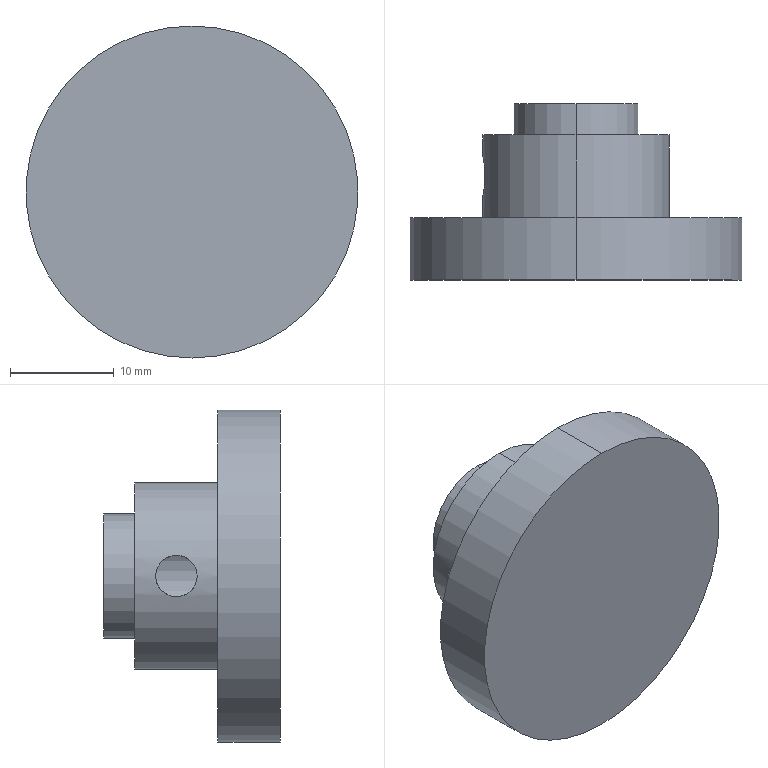Part | SolidWorks | features ICE 1, Revolution 1 | 1 solid | 15 faces | box 32 x 17 x 32 mm | volume 6483 mm3 | cylinder 10 | plane 5 | commonest cylinder face diameters 4 x2 8 x2 12 x2 18 x2 32 x2
STEP:
#1=CARTESIAN_POINT('',(-8.775,-3.306,-2.));
#2=VERTEX_POINT('',#1);
#3=CARTESIAN_POINT('',(-8.775,-3.306,2.));
#4=VERTEX_POINT('',#3);
#5=CARTESIAN_POINT('',(-8.775,-3.306,-2.));
#6=CARTESIAN_POINT('',(-8.775,-3.439,-2.));
#7=CARTESIAN_POINT('',(-8.778,-3.569,-1.987));
#8=CARTESIAN_POINT('',(-8.789,-3.826,-1.936));
#9=CARTESIAN_POINT('',(-8.798,-3.953,-1.897));
#10=CARTESIAN_POINT('',(-8.819,-4.195,-1.797));
#11=CARTESIAN_POINT('',(-8.831,-4.309,-1.735));
#12=CARTESIAN_POINT('',(-8.859,-4.527,-1.59));
#13=CARTESIAN_POINT('',(-8.874,-4.629,-1.506));
#14=CARTESIAN_POINT('',(-8.918,-4.905,-1.23));
#15=CARTESIAN_POINT('',(-8.947,-5.054,-1.007));
#16=CARTESIAN_POINT('',(-8.978,-5.203,-0.6467));
#17=CARTESIAN_POINT('',(-8.986,-5.242,-0.5202));
#18=CARTESIAN_POINT('',(-8.997,-5.294,-0.2618));
#19=CARTESIAN_POINT('',(-9.,-5.306,-0.1317));
#20=CARTESIAN_POINT('',(-9.,-5.306,0.1301));
#21=CARTESIAN_POINT('',(-8.997,-5.293,0.2631));
#22=CARTESIAN_POINT('',(-8.986,-5.242,0.52));
#23=CARTESIAN_POINT('',(-8.978,-5.204,0.6449));
#24=CARTESIAN_POINT('',(-8.947,-5.053,1.009));
#25=CARTESIAN_POINT('',(-8.918,-4.906,1.229));
#26=CARTESIAN_POINT('',(-8.873,-4.628,1.507));
#27=CARTESIAN_POINT('',(-8.859,-4.527,1.59));
#28=CARTESIAN_POINT('',(-8.832,-4.311,1.734));
#29=CARTESIAN_POINT('',(-8.819,-4.194,1.797));
#30=CARTESIAN_POINT('',(-8.798,-3.952,1.897));
#31=CARTESIAN_POINT('',(-8.789,-3.827,1.935));
#32=CARTESIAN_POINT('',(-8.778,-3.57,1.987));
#33=CARTESIAN_POINT('',(-8.775,-3.437,2.));
#34=CARTESIAN_POINT('',(-8.775,-3.306,2.));
#35=B_SPLINE_CURVE_WITH_KNOTS('',3,(#5,#6,#7,#8,#9,#10,#11,#12,#13,#14,#15,#16,#17,#18,#19,#20,#21,#22,#23,#24,#25,#26,#27,#28,#29,#30,#31,#32,#33,#34),.UNSPECIFIED.,.F.,.F.,(4,2,2,2,2,2,2,2,2,2,2,2,2,2,4),(0.,0.000392,0.0007841,0.001176,0.001568,0.002352,0.002744,0.003136,0.003528,0.00392,0.004704,0.005096,0.005488,0.00588,0.006273),.UNSPECIFIED.);
#36=EDGE_CURVE('',#2,#4,#35,.T.);
#37=ORIENTED_EDGE('',*,*,#36,.T.);
#38=CARTESIAN_POINT('',(-3.464,-3.306,2.));
#39=VERTEX_POINT('',#38);
#40=CARTESIAN_POINT('',(-10.,-3.306,2.));
#41=DIRECTION('',(1.,0.,0.));
#42=VECTOR('',#41,1000.);
#43=LINE('',#40,#42);
#44=EDGE_CURVE('',#4,#39,#43,.T.);
#45=ORIENTED_EDGE('',*,*,#44,.T.);
#46=CARTESIAN_POINT('',(-3.464,-3.306,-2.));
#47=VERTEX_POINT('',#46);
#48=CARTESIAN_POINT('',(-3.464,-3.306,2.));
#49=CARTESIAN_POINT('',(-3.464,-3.439,2.));
#50=CARTESIAN_POINT('',(-3.472,-3.574,1.986));
#51=CARTESIAN_POINT('',(-3.501,-3.833,1.934));
#52=CARTESIAN_POINT('',(-3.523,-3.958,1.895));
#53=CARTESIAN_POINT('',(-3.576,-4.201,1.794));
#54=CARTESIAN_POINT('',(-3.606,-4.315,1.732));
#55=CARTESIAN_POINT('',(-3.672,-4.529,1.588));
#56=CARTESIAN_POINT('',(-3.707,-4.63,1.505));
#57=CARTESIAN_POINT('',(-3.776,-4.811,1.324));
#58=CARTESIAN_POINT('',(-3.81,-4.893,1.225));
#59=CARTESIAN_POINT('',(-3.872,-5.038,1.01));
#60=CARTESIAN_POINT('',(-3.901,-5.1,0.8936));
#61=CARTESIAN_POINT('',(-3.972,-5.251,0.5337));
#62=CARTESIAN_POINT('',(-4.,-5.306,0.2665));
#63=CARTESIAN_POINT('',(-4.,-5.307,-0.1307));
#64=CARTESIAN_POINT('',(-3.993,-5.293,-0.265));
#65=CARTESIAN_POINT('',(-3.967,-5.241,-0.5254));
#66=CARTESIAN_POINT('',(-3.949,-5.202,-0.651));
#67=CARTESIAN_POINT('',(-3.877,-5.05,-1.015));
#68=CARTESIAN_POINT('',(-3.81,-4.902,-1.233));
#69=CARTESIAN_POINT('',(-3.707,-4.628,-1.507));
#70=CARTESIAN_POINT('',(-3.672,-4.529,-1.588));
#71=CARTESIAN_POINT('',(-3.607,-4.316,-1.732));
#72=CARTESIAN_POINT('',(-3.575,-4.2,-1.794));
#73=CARTESIAN_POINT('',(-3.523,-3.96,-1.895));
#74=CARTESIAN_POINT('',(-3.502,-3.835,-1.933));
#75=CARTESIAN_POINT('',(-3.472,-3.576,-1.986));
#76=CARTESIAN_POINT('',(-3.464,-3.441,-2.));
#77=CARTESIAN_POINT('',(-3.464,-3.306,-2.));
#78=B_SPLINE_CURVE_WITH_KNOTS('',3,(#48,#49,#50,#51,#52,#53,#54,#55,#56,#57,#58,#59,#60,#61,#62,#63,#64,#65,#66,#67,#68,#69,#70,#71,#72,#73,#74,#75,#76,#77),.UNSPECIFIED.,.F.,.F.,(4,2,2,2,2,2,2,2,2,2,2,2,2,2,4),(0.006361,0.006758,0.007155,0.007552,0.007949,0.008346,0.008742,0.009536,0.009933,0.01033,0.01112,0.01152,0.01192,0.01231,0.01271),.UNSPECIFIED.);
#79=EDGE_CURVE('',#39,#47,#78,.T.);
#80=ORIENTED_EDGE('',*,*,#79,.T.);
#81=CARTESIAN_POINT('',(-10.,-3.306,-2.));
#82=DIRECTION('',(1.,0.,0.));
#83=VECTOR('',#82,1000.);
#84=LINE('',#81,#83);
#85=EDGE_CURVE('',#2,#47,#84,.T.);
#86=ORIENTED_EDGE('',*,*,#85,.F.);
#87=EDGE_LOOP('',(#37,#45,#80,#86));
#88=FACE_OUTER_BOUND('',#87,.T.);
#89=CARTESIAN_POINT('',(-10.,-3.306,0.));
#90=DIRECTION('',(1.,0.,0.));
#91=DIRECTION('',(0.,0.,-1.));
#92=AXIS2_PLACEMENT_3D('',#89,#90,#91);
#93=CYLINDRICAL_SURFACE('',#92,2.);
#94=ADVANCED_FACE('',(#88),#93,.F.);
#95=CARTESIAN_POINT('',(0.,3.694,-6.));
#96=VERTEX_POINT('',#95);
#97=CARTESIAN_POINT('',(0.,3.694,6.));
#98=VERTEX_POINT('',#97);
#99=CARTESIAN_POINT('',(0.,3.694,0.));
#100=DIRECTION('',(0.,-1.,0.));
#101=DIRECTION('',(0.,0.,-1.));
#102=AXIS2_PLACEMENT_3D('',#99,#100,#101);
#103=CIRCLE('',#102,6.);
#104=EDGE_CURVE('',#96,#98,#103,.T.);
#105=ORIENTED_EDGE('',*,*,#104,.T.);
#106=CARTESIAN_POINT('',(0.,0.6936,6.));
#107=VERTEX_POINT('',#106);
#108=CARTESIAN_POINT('',(0.,0.,6.));
#109=DIRECTION('',(0.,-1.,0.));
#110=VECTOR('',#109,1000.);
#111=LINE('',#108,#110);
#112=EDGE_CURVE('',#98,#107,#111,.T.);
#113=ORIENTED_EDGE('',*,*,#112,.T.);
#114=CARTESIAN_POINT('',(0.,0.6936,-6.));
#115=VERTEX_POINT('',#114);
#116=CARTESIAN_POINT('',(0.,0.6936,0.));
#117=DIRECTION('',(0.,-1.,0.));
#118=DIRECTION('',(0.,0.,-1.));
#119=AXIS2_PLACEMENT_3D('',#116,#117,#118);
#120=CIRCLE('',#119,6.);
#121=EDGE_CURVE('',#115,#107,#120,.T.);
#122=ORIENTED_EDGE('',*,*,#121,.F.);
#123=CARTESIAN_POINT('',(0.,0.,-6.));
#124=DIRECTION('',(0.,-1.,0.));
#125=VECTOR('',#124,1000.);
#126=LINE('',#123,#125);
#127=EDGE_CURVE('',#96,#115,#126,.T.);
#128=ORIENTED_EDGE('',*,*,#127,.F.);
#129=EDGE_LOOP('',(#105,#113,#122,#128));
#130=FACE_OUTER_BOUND('',#129,.T.);
#131=CARTESIAN_POINT('',(0.,0.,0.));
#132=DIRECTION('',(0.,-1.,0.));
#133=DIRECTION('',(0.,0.,-1.));
#134=AXIS2_PLACEMENT_3D('',#131,#132,#133);
#135=CYLINDRICAL_SURFACE('',#134,6.);
#136=ADVANCED_FACE('',(#130),#135,.T.);
#137=CARTESIAN_POINT('',(0.,0.6936,-9.));
#138=VERTEX_POINT('',#137);
#139=CARTESIAN_POINT('',(0.,0.6936,9.));
#140=VERTEX_POINT('',#139);
#141=CARTESIAN_POINT('',(0.,0.6936,0.));
#142=DIRECTION('',(0.,-1.,0.));
#143=DIRECTION('',(0.,0.,-1.));
#144=AXIS2_PLACEMENT_3D('',#141,#142,#143);
#145=CIRCLE('',#144,9.);
#146=EDGE_CURVE('',#138,#140,#145,.T.);
#147=ORIENTED_EDGE('',*,*,#146,.T.);
#148=CARTESIAN_POINT('',(0.,-7.306,9.));
#149=VERTEX_POINT('',#148);
#150=CARTESIAN_POINT('',(0.,0.,9.));
#151=DIRECTION('',(0.,-1.,0.));
#152=VECTOR('',#151,1000.);
#153=LINE('',#150,#152);
#154=EDGE_CURVE('',#140,#149,#153,.T.);
#155=ORIENTED_EDGE('',*,*,#154,.T.);
#156=CARTESIAN_POINT('',(0.,-7.306,-9.));
#157=VERTEX_POINT('',#156);
#158=CARTESIAN_POINT('',(0.,-7.306,0.));
#159=DIRECTION('',(0.,-1.,0.));
#160=DIRECTION('',(0.,0.,-1.));
#161=AXIS2_PLACEMENT_3D('',#158,#159,#160);
#162=CIRCLE('',#161,9.);
#163=EDGE_CURVE('',#157,#149,#162,.T.);
#164=ORIENTED_EDGE('',*,*,#163,.F.);
#165=CARTESIAN_POINT('',(0.,0.,-9.));
#166=DIRECTION('',(0.,-1.,0.));
#167=VECTOR('',#166,1000.);
#168=LINE('',#165,#167);
#169=EDGE_CURVE('',#138,#157,#168,.T.);
#170=ORIENTED_EDGE('',*,*,#169,.F.);
#171=EDGE_LOOP('',(#147,#155,#164,#170));
#172=FACE_OUTER_BOUND('',#171,.T.);
#173=CARTESIAN_POINT('',(0.,0.,0.));
#174=DIRECTION('',(0.,-1.,0.));
#175=DIRECTION('',(0.,0.,-1.));
#176=AXIS2_PLACEMENT_3D('',#173,#174,#175);
#177=CYLINDRICAL_SURFACE('',#176,9.);
#178=ADVANCED_FACE('',(#172),#177,.T.);
#179=CARTESIAN_POINT('',(0.,-7.306,-16.));
#180=VERTEX_POINT('',#179);
#181=CARTESIAN_POINT('',(0.,-7.306,16.));
#182=VERTEX_POINT('',#181);
#183=CARTESIAN_POINT('',(0.,-7.306,0.));
#184=DIRECTION('',(0.,-1.,0.));
#185=DIRECTION('',(0.,0.,-1.));
#186=AXIS2_PLACEMENT_3D('',#183,#184,#185);
#187=CIRCLE('',#186,16.);
#188=EDGE_CURVE('',#180,#182,#187,.T.);
#189=ORIENTED_EDGE('',*,*,#188,.T.);
#190=CARTESIAN_POINT('',(0.,-13.306,16.));
#191=VERTEX_POINT('',#190);
#192=CARTESIAN_POINT('',(0.,0.,16.));
#193=DIRECTION('',(0.,-1.,0.));
#194=VECTOR('',#193,1000.);
#195=LINE('',#192,#194);
#196=EDGE_CURVE('',#182,#191,#195,.T.);
#197=ORIENTED_EDGE('',*,*,#196,.T.);
#198=CARTESIAN_POINT('',(0.,-13.306,-16.));
#199=VERTEX_POINT('',#198);
#200=CARTESIAN_POINT('',(0.,-13.306,0.));
#201=DIRECTION('',(0.,-1.,0.));
#202=DIRECTION('',(0.,0.,-1.));
#203=AXIS2_PLACEMENT_3D('',#200,#201,#202);
#204=CIRCLE('',#203,16.);
#205=EDGE_CURVE('',#199,#191,#204,.T.);
#206=ORIENTED_EDGE('',*,*,#205,.F.);
#207=CARTESIAN_POINT('',(0.,0.,-16.));
#208=DIRECTION('',(0.,-1.,0.));
#209=VECTOR('',#208,1000.);
#210=LINE('',#207,#209);
#211=EDGE_CURVE('',#180,#199,#210,.T.);
#212=ORIENTED_EDGE('',*,*,#211,.F.);
#213=EDGE_LOOP('',(#189,#197,#206,#212));
#214=FACE_OUTER_BOUND('',#213,.T.);
#215=CARTESIAN_POINT('',(0.,0.,0.));
#216=DIRECTION('',(0.,-1.,0.));
#217=DIRECTION('',(0.,0.,-1.));
#218=AXIS2_PLACEMENT_3D('',#215,#216,#217);
#219=CYLINDRICAL_SURFACE('',#218,16.);
#220=ADVANCED_FACE('',(#214),#219,.T.);
#221=CARTESIAN_POINT('',(-3.464,-3.306,-2.));
#222=CARTESIAN_POINT('',(-3.464,-3.172,-2.));
#223=CARTESIAN_POINT('',(-3.472,-3.04,-1.987));
#224=CARTESIAN_POINT('',(-3.501,-2.781,-1.934));
#225=CARTESIAN_POINT('',(-3.523,-2.653,-1.895));
#226=CARTESIAN_POINT('',(-3.602,-2.292,-1.743));
#227=CARTESIAN_POINT('',(-3.673,-2.074,-1.596));
#228=CARTESIAN_POINT('',(-3.81,-1.711,-1.233));
#229=CARTESIAN_POINT('',(-3.877,-1.563,-1.014));
#230=CARTESIAN_POINT('',(-3.948,-1.412,-0.6539));
#231=CARTESIAN_POINT('',(-3.967,-1.372,-0.5256));
#232=CARTESIAN_POINT('',(-3.993,-1.32,-0.2661));
#233=CARTESIAN_POINT('',(-4.,-1.307,-0.1346));
#234=CARTESIAN_POINT('',(-4.,-1.306,0.132));
#235=CARTESIAN_POINT('',(-3.993,-1.32,0.2666));
#236=CARTESIAN_POINT('',(-3.967,-1.372,0.5257));
#237=CARTESIAN_POINT('',(-3.948,-1.411,0.653));
#238=CARTESIAN_POINT('',(-3.9,-1.513,0.8959));
#239=CARTESIAN_POINT('',(-3.872,-1.575,1.01));
#240=CARTESIAN_POINT('',(-3.809,-1.72,1.225));
#241=CARTESIAN_POINT('',(-3.775,-1.804,1.326));
#242=CARTESIAN_POINT('',(-3.672,-2.076,1.598));
#243=CARTESIAN_POINT('',(-3.601,-2.295,1.745));
#244=CARTESIAN_POINT('',(-3.523,-2.654,1.895));
#245=CARTESIAN_POINT('',(-3.501,-2.781,1.934));
#246=CARTESIAN_POINT('',(-3.472,-3.042,1.987));
#247=CARTESIAN_POINT('',(-3.464,-3.174,2.));
#248=CARTESIAN_POINT('',(-3.464,-3.306,2.));
#249=B_SPLINE_CURVE_WITH_KNOTS('',3,(#221,#222,#223,#224,#225,#226,#227,#228,#229,#230,#231,#232,#233,#234,#235,#236,#237,#238,#239,#240,#241,#242,#243,#244,#245,#246,#247,#248),.UNSPECIFIED.,.F.,.F.,(4,2,2,2,2,2,2,2,2,2,2,2,2,4),(0.,0.0003976,0.0007951,0.00159,0.002385,0.002783,0.003181,0.003578,0.003976,0.004373,0.004771,0.005566,0.005964,0.006361),.UNSPECIFIED.);
#250=EDGE_CURVE('',#47,#39,#249,.T.);
#251=ORIENTED_EDGE('',*,*,#250,.F.);
#252=ORIENTED_EDGE('',*,*,#79,.F.);
#253=EDGE_LOOP('',(#251,#252));
#254=FACE_BOUND('',#253,.T.);
#255=CARTESIAN_POINT('',(0.,3.694,4.));
#256=VERTEX_POINT('',#255);
#257=CARTESIAN_POINT('',(0.,3.694,-4.));
#258=VERTEX_POINT('',#257);
#259=CARTESIAN_POINT('',(0.,3.694,0.));
#260=DIRECTION('',(0.,-1.,0.));
#261=DIRECTION('',(0.,0.,-1.));
#262=AXIS2_PLACEMENT_3D('',#259,#260,#261);
#263=CIRCLE('',#262,4.);
#264=EDGE_CURVE('',#256,#258,#263,.T.);
#265=ORIENTED_EDGE('',*,*,#264,.F.);
#266=CARTESIAN_POINT('',(0.,-9.306,4.));
#267=VERTEX_POINT('',#266);
#268=CARTESIAN_POINT('',(0.,0.,4.));
#269=DIRECTION('',(0.,-1.,0.));
#270=VECTOR('',#269,1000.);
#271=LINE('',#268,#270);
#272=EDGE_CURVE('',#256,#267,#271,.T.);
#273=ORIENTED_EDGE('',*,*,#272,.T.);
#274=CARTESIAN_POINT('',(0.,-9.306,-4.));
#275=VERTEX_POINT('',#274);
#276=CARTESIAN_POINT('',(0.,-9.306,0.));
#277=DIRECTION('',(0.,-1.,0.));
#278=DIRECTION('',(0.,0.,-1.));
#279=AXIS2_PLACEMENT_3D('',#276,#277,#278);
#280=CIRCLE('',#279,4.);
#281=EDGE_CURVE('',#267,#275,#280,.T.);
#282=ORIENTED_EDGE('',*,*,#281,.T.);
#283=CARTESIAN_POINT('',(0.,0.,-4.));
#284=DIRECTION('',(0.,-1.,0.));
#285=VECTOR('',#284,1000.);
#286=LINE('',#283,#285);
#287=EDGE_CURVE('',#258,#275,#286,.T.);
#288=ORIENTED_EDGE('',*,*,#287,.F.);
#289=EDGE_LOOP('',(#265,#273,#282,#288));
#290=FACE_OUTER_BOUND('',#289,.T.);
#291=CARTESIAN_POINT('',(0.,0.,0.));
#292=DIRECTION('',(0.,-1.,0.));
#293=DIRECTION('',(0.,0.,-1.));
#294=AXIS2_PLACEMENT_3D('',#291,#292,#293);
#295=CYLINDRICAL_SURFACE('',#294,4.);
#296=ADVANCED_FACE('',(#254,#290),#295,.F.);
#297=CARTESIAN_POINT('',(0.,3.694,0.));
#298=DIRECTION('',(0.,-1.,0.));
#299=DIRECTION('',(0.,0.,-1.));
#300=AXIS2_PLACEMENT_3D('',#297,#298,#299);
#301=CIRCLE('',#300,4.);
#302=EDGE_CURVE('',#258,#256,#301,.T.);
#303=ORIENTED_EDGE('',*,*,#302,.T.);
#304=ORIENTED_EDGE('',*,*,#264,.T.);
#305=EDGE_LOOP('',(#303,#304));
#306=FACE_BOUND('',#305,.T.);
#307=ORIENTED_EDGE('',*,*,#104,.F.);
#308=CARTESIAN_POINT('',(0.,3.694,0.));
#309=DIRECTION('',(0.,-1.,0.));
#310=DIRECTION('',(0.,0.,-1.));
#311=AXIS2_PLACEMENT_3D('',#308,#309,#310);
#312=CIRCLE('',#311,6.);
#313=EDGE_CURVE('',#98,#96,#312,.T.);
#314=ORIENTED_EDGE('',*,*,#313,.F.);
#315=EDGE_LOOP('',(#307,#314));
#316=FACE_OUTER_BOUND('',#315,.T.);
#317=CARTESIAN_POINT('',(6.,3.694,0.));
#318=DIRECTION('',(0.,1.,0.));
#319=DIRECTION('',(0.,0.,1.));
#320=AXIS2_PLACEMENT_3D('',#317,#318,#319);
#321=PLANE('',#320);
#322=ADVANCED_FACE('',(#306,#316),#321,.T.);
#323=ORIENTED_EDGE('',*,*,#272,.F.);
#324=ORIENTED_EDGE('',*,*,#302,.F.);
#325=ORIENTED_EDGE('',*,*,#287,.T.);
#326=CARTESIAN_POINT('',(0.,-9.306,0.));
#327=DIRECTION('',(0.,-1.,0.));
#328=DIRECTION('',(0.,0.,-1.));
#329=AXIS2_PLACEMENT_3D('',#326,#327,#328);
#330=CIRCLE('',#329,4.);
#331=EDGE_CURVE('',#275,#267,#330,.T.);
#332=ORIENTED_EDGE('',*,*,#331,.T.);
#333=EDGE_LOOP('',(#323,#324,#325,#332));
#334=FACE_OUTER_BOUND('',#333,.T.);
#335=CARTESIAN_POINT('',(0.,0.,0.));
#336=DIRECTION('',(0.,-1.,0.));
#337=DIRECTION('',(0.,0.,-1.));
#338=AXIS2_PLACEMENT_3D('',#335,#336,#337);
#339=CYLINDRICAL_SURFACE('',#338,4.);
#340=ADVANCED_FACE('',(#334),#339,.F.);
#341=ORIENTED_EDGE('',*,*,#331,.F.);
#342=ORIENTED_EDGE('',*,*,#281,.F.);
#343=EDGE_LOOP('',(#341,#342));
#344=FACE_OUTER_BOUND('',#343,.T.);
#345=CARTESIAN_POINT('',(4.,-9.306,0.));
#346=DIRECTION('',(0.,1.,0.));
#347=DIRECTION('',(0.,0.,1.));
#348=AXIS2_PLACEMENT_3D('',#345,#346,#347);
#349=PLANE('',#348);
#350=ADVANCED_FACE('',(#344),#349,.T.);
#351=ORIENTED_EDGE('',*,*,#205,.T.);
#352=CARTESIAN_POINT('',(0.,-13.306,0.));
#353=DIRECTION('',(0.,-1.,0.));
#354=DIRECTION('',(0.,0.,-1.));
#355=AXIS2_PLACEMENT_3D('',#352,#353,#354);
#356=CIRCLE('',#355,16.);
#357=EDGE_CURVE('',#191,#199,#356,.T.);
#358=ORIENTED_EDGE('',*,*,#357,.T.);
#359=EDGE_LOOP('',(#351,#358));
#360=FACE_OUTER_BOUND('',#359,.T.);
#361=CARTESIAN_POINT('',(16.,-13.306,0.));
#362=DIRECTION('',(0.,-1.,0.));
#363=DIRECTION('',(0.,0.,-1.));
#364=AXIS2_PLACEMENT_3D('',#361,#362,#363);
#365=PLANE('',#364);
#366=ADVANCED_FACE('',(#360),#365,.T.);
#367=ORIENTED_EDGE('',*,*,#196,.F.);
#368=CARTESIAN_POINT('',(0.,-7.306,0.));
#369=DIRECTION('',(0.,-1.,0.));
#370=DIRECTION('',(0.,0.,-1.));
#371=AXIS2_PLACEMENT_3D('',#368,#369,#370);
#372=CIRCLE('',#371,16.);
#373=EDGE_CURVE('',#182,#180,#372,.T.);
#374=ORIENTED_EDGE('',*,*,#373,.T.);
#375=ORIENTED_EDGE('',*,*,#211,.T.);
#376=ORIENTED_EDGE('',*,*,#357,.F.);
#377=EDGE_LOOP('',(#367,#374,#375,#376));
#378=FACE_OUTER_BOUND('',#377,.T.);
#379=CARTESIAN_POINT('',(0.,0.,0.));
#380=DIRECTION('',(0.,-1.,0.));
#381=DIRECTION('',(0.,0.,-1.));
#382=AXIS2_PLACEMENT_3D('',#379,#380,#381);
#383=CYLINDRICAL_SURFACE('',#382,16.);
#384=ADVANCED_FACE('',(#378),#383,.T.);
#385=ORIENTED_EDGE('',*,*,#163,.T.);
#386=CARTESIAN_POINT('',(0.,-7.306,0.));
#387=DIRECTION('',(0.,-1.,0.));
#388=DIRECTION('',(0.,0.,-1.));
#389=AXIS2_PLACEMENT_3D('',#386,#387,#388);
#390=CIRCLE('',#389,9.);
#391=EDGE_CURVE('',#149,#157,#390,.T.);
#392=ORIENTED_EDGE('',*,*,#391,.T.);
#393=EDGE_LOOP('',(#385,#392));
#394=FACE_BOUND('',#393,.T.);
#395=ORIENTED_EDGE('',*,*,#188,.F.);
#396=ORIENTED_EDGE('',*,*,#373,.F.);
#397=EDGE_LOOP('',(#395,#396));
#398=FACE_OUTER_BOUND('',#397,.T.);
#399=CARTESIAN_POINT('',(9.,-7.306,0.));
#400=DIRECTION('',(0.,1.,0.));
#401=DIRECTION('',(0.,0.,1.));
#402=AXIS2_PLACEMENT_3D('',#399,#400,#401);
#403=PLANE('',#402);
#404=ADVANCED_FACE('',(#394,#398),#403,.T.);
#405=ORIENTED_EDGE('',*,*,#154,.F.);
#406=CARTESIAN_POINT('',(0.,0.6936,0.));
#407=DIRECTION('',(0.,-1.,0.));
#408=DIRECTION('',(0.,0.,-1.));
#409=AXIS2_PLACEMENT_3D('',#406,#407,#408);
#410=CIRCLE('',#409,9.);
#411=EDGE_CURVE('',#140,#138,#410,.T.);
#412=ORIENTED_EDGE('',*,*,#411,.T.);
#413=ORIENTED_EDGE('',*,*,#169,.T.);
#414=ORIENTED_EDGE('',*,*,#391,.F.);
#415=EDGE_LOOP('',(#405,#412,#413,#414));
#416=FACE_OUTER_BOUND('',#415,.T.);
#417=ORIENTED_EDGE('',*,*,#36,.F.);
#418=CARTESIAN_POINT('',(-8.775,-3.306,2.));
#419=CARTESIAN_POINT('',(-8.775,-3.045,2.));
#420=CARTESIAN_POINT('',(-8.787,-2.781,1.947));
#421=CARTESIAN_POINT('',(-8.819,-2.42,1.797));
#422=CARTESIAN_POINT('',(-8.831,-2.303,1.735));
#423=CARTESIAN_POINT('',(-8.859,-2.086,1.59));
#424=CARTESIAN_POINT('',(-8.873,-1.985,1.507));
#425=CARTESIAN_POINT('',(-8.903,-1.801,1.323));
#426=CARTESIAN_POINT('',(-8.918,-1.717,1.22));
#427=CARTESIAN_POINT('',(-8.944,-1.572,1.004));
#428=CARTESIAN_POINT('',(-8.957,-1.51,0.8894));
#429=CARTESIAN_POINT('',(-8.988,-1.359,0.525));
#430=CARTESIAN_POINT('',(-9.,-1.307,0.2648));
#431=CARTESIAN_POINT('',(-9.,-1.306,-0.1312));
#432=CARTESIAN_POINT('',(-8.997,-1.319,-0.2613));
#433=CARTESIAN_POINT('',(-8.986,-1.37,-0.5178));
#434=CARTESIAN_POINT('',(-8.978,-1.409,-0.6454));
#435=CARTESIAN_POINT('',(-8.957,-1.509,-0.8868));
#436=CARTESIAN_POINT('',(-8.945,-1.57,-1.002));
#437=CARTESIAN_POINT('',(-8.918,-1.716,-1.22));
#438=CARTESIAN_POINT('',(-8.903,-1.8,-1.322));
#439=CARTESIAN_POINT('',(-8.859,-2.075,-1.597));
#440=CARTESIAN_POINT('',(-8.83,-2.297,-1.746));
#441=CARTESIAN_POINT('',(-8.798,-2.658,-1.896));
#442=CARTESIAN_POINT('',(-8.789,-2.785,-1.935));
#443=CARTESIAN_POINT('',(-8.778,-3.043,-1.987));
#444=CARTESIAN_POINT('',(-8.775,-3.174,-2.));
#445=CARTESIAN_POINT('',(-8.775,-3.306,-2.));
#446=B_SPLINE_CURVE_WITH_KNOTS('',3,(#418,#419,#420,#421,#422,#423,#424,#425,#426,#427,#428,#429,#430,#431,#432,#433,#434,#435,#436,#437,#438,#439,#440,#441,#442,#443,#444,#445),.UNSPECIFIED.,.F.,.F.,(4,2,2,2,2,2,2,2,2,2,2,2,2,4),(0.006273,0.007056,0.007448,0.00784,0.008232,0.008624,0.009408,0.0098,0.01019,0.01058,0.01098,0.01176,0.01215,0.01254),.UNSPECIFIED.);
#447=EDGE_CURVE('',#4,#2,#446,.T.);
#448=ORIENTED_EDGE('',*,*,#447,.F.);
#449=EDGE_LOOP('',(#417,#448));
#450=FACE_BOUND('',#449,.T.);
#451=CARTESIAN_POINT('',(0.,0.,0.));
#452=DIRECTION('',(0.,-1.,0.));
#453=DIRECTION('',(0.,0.,-1.));
#454=AXIS2_PLACEMENT_3D('',#451,#452,#453);
#455=CYLINDRICAL_SURFACE('',#454,9.);
#456=ADVANCED_FACE('',(#416,#450),#455,.T.);
#457=ORIENTED_EDGE('',*,*,#121,.T.);
#458=CARTESIAN_POINT('',(0.,0.6936,0.));
#459=DIRECTION('',(0.,-1.,0.));
#460=DIRECTION('',(0.,0.,-1.));
#461=AXIS2_PLACEMENT_3D('',#458,#459,#460);
#462=CIRCLE('',#461,6.);
#463=EDGE_CURVE('',#107,#115,#462,.T.);
#464=ORIENTED_EDGE('',*,*,#463,.T.);
#465=EDGE_LOOP('',(#457,#464));
#466=FACE_BOUND('',#465,.T.);
#467=ORIENTED_EDGE('',*,*,#146,.F.);
#468=ORIENTED_EDGE('',*,*,#411,.F.);
#469=EDGE_LOOP('',(#467,#468));
#470=FACE_OUTER_BOUND('',#469,.T.);
#471=CARTESIAN_POINT('',(6.,0.6936,0.));
#472=DIRECTION('',(0.,1.,0.));
#473=DIRECTION('',(0.,0.,1.));
#474=AXIS2_PLACEMENT_3D('',#471,#472,#473);
#475=PLANE('',#474);
#476=ADVANCED_FACE('',(#466,#470),#475,.T.);
#477=ORIENTED_EDGE('',*,*,#112,.F.);
#478=ORIENTED_EDGE('',*,*,#313,.T.);
#479=ORIENTED_EDGE('',*,*,#127,.T.);
#480=ORIENTED_EDGE('',*,*,#463,.F.);
#481=EDGE_LOOP('',(#477,#478,#479,#480));
#482=FACE_OUTER_BOUND('',#481,.T.);
#483=CARTESIAN_POINT('',(0.,0.,0.));
#484=DIRECTION('',(0.,-1.,0.));
#485=DIRECTION('',(0.,0.,-1.));
#486=AXIS2_PLACEMENT_3D('',#483,#484,#485);
#487=CYLINDRICAL_SURFACE('',#486,6.);
#488=ADVANCED_FACE('',(#482),#487,.T.);
#489=ORIENTED_EDGE('',*,*,#44,.F.);
#490=ORIENTED_EDGE('',*,*,#447,.T.);
#491=ORIENTED_EDGE('',*,*,#85,.T.);
#492=ORIENTED_EDGE('',*,*,#250,.T.);
#493=EDGE_LOOP('',(#489,#490,#491,#492));
#494=FACE_OUTER_BOUND('',#493,.T.);
#495=CARTESIAN_POINT('',(-10.,-3.306,0.));
#496=DIRECTION('',(1.,0.,0.));
#497=DIRECTION('',(0.,0.,-1.));
#498=AXIS2_PLACEMENT_3D('',#495,#496,#497);
#499=CYLINDRICAL_SURFACE('',#498,2.);
#500=ADVANCED_FACE('',(#494),#499,.F.);
#501=CLOSED_SHELL('',(#94,#136,#178,#220,#296,#322,#340,#350,#366,#384,#404,#456,#476,#488,#500));
#502=MANIFOLD_SOLID_BREP('',#501);
#503=CARTESIAN_POINT('',(0.,0.,0.));
#504=DIRECTION('',(0.,0.,1.));
#505=DIRECTION('',(1.,0.,0.));
#506=AXIS2_PLACEMENT_3D('',#503,#504,#505);
#507=(LENGTH_UNIT()NAMED_UNIT(*)SI_UNIT(.MILLI.,.METRE.));
#508=UNCERTAINTY_MEASURE_WITH_UNIT(LENGTH_MEASURE(0.00001),#507,'','');
#509=(NAMED_UNIT(*)PLANE_ANGLE_UNIT()SI_UNIT($,.RADIAN.));
#510=(NAMED_UNIT(*)SI_UNIT($,.STERADIAN.)SOLID_ANGLE_UNIT());
#511=(GEOMETRIC_REPRESENTATION_CONTEXT(3)GLOBAL_UNCERTAINTY_ASSIGNED_CONTEXT((#508))GLOBAL_UNIT_ASSIGNED_CONTEXT((#507,#509,#510))REPRESENTATION_CONTEXT('',''));
#512=ADVANCED_BREP_SHAPE_REPRESENTATION('',(#502,#506),#511);